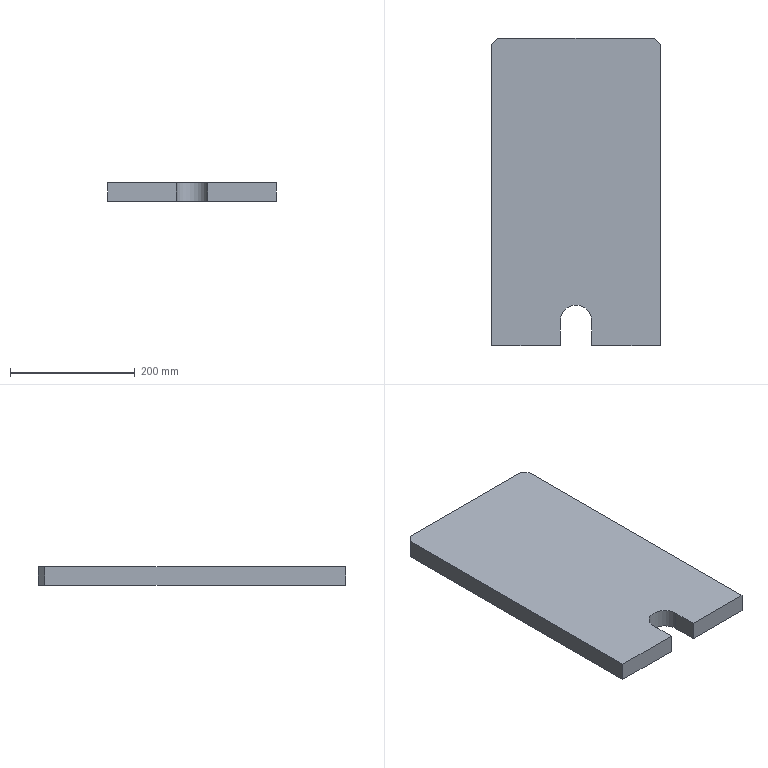Part | SolidWorks | features Extrusion 1 | 1 solid | 12 faces | box 270 x 492 x 30 mm | volume 3892748 mm3 | plane 11 | cylinder 1 | commonest cylinder face diameters 50 x1
STEP:
#1=CARTESIAN_POINT('',(0.,482.,0.));
#2=VERTEX_POINT('',#1);
#3=CARTESIAN_POINT('',(0.,0.,0.));
#4=VERTEX_POINT('',#3);
#5=CARTESIAN_POINT('',(0.,0.,0.));
#6=DIRECTION('',(0.,-1.,0.));
#7=VECTOR('',#6,1000.);
#8=LINE('',#5,#7);
#9=EDGE_CURVE('',#2,#4,#8,.T.);
#10=ORIENTED_EDGE('',*,*,#9,.T.);
#11=CARTESIAN_POINT('',(0.,0.,30.));
#12=VERTEX_POINT('',#11);
#13=CARTESIAN_POINT('',(0.,0.,30.));
#14=DIRECTION('',(0.,0.,-1.));
#15=VECTOR('',#14,1000.);
#16=LINE('',#13,#15);
#17=EDGE_CURVE('',#12,#4,#16,.T.);
#18=ORIENTED_EDGE('',*,*,#17,.F.);
#19=CARTESIAN_POINT('',(0.,482.,30.));
#20=VERTEX_POINT('',#19);
#21=CARTESIAN_POINT('',(0.,0.,30.));
#22=DIRECTION('',(0.,-1.,0.));
#23=VECTOR('',#22,1000.);
#24=LINE('',#21,#23);
#25=EDGE_CURVE('',#20,#12,#24,.T.);
#26=ORIENTED_EDGE('',*,*,#25,.F.);
#27=CARTESIAN_POINT('',(0.,482.,30.));
#28=DIRECTION('',(0.,0.,-1.));
#29=VECTOR('',#28,1000.);
#30=LINE('',#27,#29);
#31=EDGE_CURVE('',#20,#2,#30,.T.);
#32=ORIENTED_EDGE('',*,*,#31,.T.);
#33=EDGE_LOOP('',(#10,#18,#26,#32));
#34=FACE_OUTER_BOUND('',#33,.T.);
#35=CARTESIAN_POINT('',(0.,0.,30.));
#36=DIRECTION('',(1.,0.,0.));
#37=DIRECTION('',(0.,0.,-1.));
#38=AXIS2_PLACEMENT_3D('',#35,#36,#37);
#39=PLANE('',#38);
#40=ADVANCED_FACE('',(#34),#39,.F.);
#41=CARTESIAN_POINT('',(110.,0.,0.));
#42=VERTEX_POINT('',#41);
#43=CARTESIAN_POINT('',(0.,0.,0.));
#44=DIRECTION('',(1.,0.,0.));
#45=VECTOR('',#44,1000.);
#46=LINE('',#43,#45);
#47=EDGE_CURVE('',#4,#42,#46,.T.);
#48=ORIENTED_EDGE('',*,*,#47,.T.);
#49=CARTESIAN_POINT('',(110.,0.,30.));
#50=VERTEX_POINT('',#49);
#51=CARTESIAN_POINT('',(110.,0.,30.));
#52=DIRECTION('',(0.,0.,-1.));
#53=VECTOR('',#52,1000.);
#54=LINE('',#51,#53);
#55=EDGE_CURVE('',#50,#42,#54,.T.);
#56=ORIENTED_EDGE('',*,*,#55,.F.);
#57=CARTESIAN_POINT('',(0.,0.,30.));
#58=DIRECTION('',(1.,0.,0.));
#59=VECTOR('',#58,1000.);
#60=LINE('',#57,#59);
#61=EDGE_CURVE('',#12,#50,#60,.T.);
#62=ORIENTED_EDGE('',*,*,#61,.F.);
#63=ORIENTED_EDGE('',*,*,#17,.T.);
#64=EDGE_LOOP('',(#48,#56,#62,#63));
#65=FACE_OUTER_BOUND('',#64,.T.);
#66=CARTESIAN_POINT('',(0.,0.,30.));
#67=DIRECTION('',(0.,1.,0.));
#68=DIRECTION('',(0.,0.,1.));
#69=AXIS2_PLACEMENT_3D('',#66,#67,#68);
#70=PLANE('',#69);
#71=ADVANCED_FACE('',(#65),#70,.F.);
#72=CARTESIAN_POINT('',(110.,40.,0.));
#73=VERTEX_POINT('',#72);
#74=CARTESIAN_POINT('',(110.,0.,0.));
#75=DIRECTION('',(0.,1.,0.));
#76=VECTOR('',#75,1000.);
#77=LINE('',#74,#76);
#78=EDGE_CURVE('',#42,#73,#77,.T.);
#79=ORIENTED_EDGE('',*,*,#78,.T.);
#80=CARTESIAN_POINT('',(110.,40.,30.));
#81=VERTEX_POINT('',#80);
#82=CARTESIAN_POINT('',(110.,40.,30.));
#83=DIRECTION('',(0.,0.,-1.));
#84=VECTOR('',#83,1000.);
#85=LINE('',#82,#84);
#86=EDGE_CURVE('',#81,#73,#85,.T.);
#87=ORIENTED_EDGE('',*,*,#86,.F.);
#88=CARTESIAN_POINT('',(110.,0.,30.));
#89=DIRECTION('',(0.,1.,0.));
#90=VECTOR('',#89,1000.);
#91=LINE('',#88,#90);
#92=EDGE_CURVE('',#50,#81,#91,.T.);
#93=ORIENTED_EDGE('',*,*,#92,.F.);
#94=ORIENTED_EDGE('',*,*,#55,.T.);
#95=EDGE_LOOP('',(#79,#87,#93,#94));
#96=FACE_OUTER_BOUND('',#95,.T.);
#97=CARTESIAN_POINT('',(110.,0.,30.));
#98=DIRECTION('',(-1.,0.,0.));
#99=DIRECTION('',(0.,0.,1.));
#100=AXIS2_PLACEMENT_3D('',#97,#98,#99);
#101=PLANE('',#100);
#102=ADVANCED_FACE('',(#96),#101,.F.);
#103=CARTESIAN_POINT('',(160.,40.,0.));
#104=VERTEX_POINT('',#103);
#105=CARTESIAN_POINT('',(135.,40.,0.));
#106=DIRECTION('',(0.,0.,-1.));
#107=DIRECTION('',(-1.,0.,0.));
#108=AXIS2_PLACEMENT_3D('',#105,#106,#107);
#109=CIRCLE('',#108,25.);
#110=EDGE_CURVE('',#73,#104,#109,.T.);
#111=ORIENTED_EDGE('',*,*,#110,.T.);
#112=CARTESIAN_POINT('',(160.,40.,30.));
#113=VERTEX_POINT('',#112);
#114=CARTESIAN_POINT('',(160.,40.,30.));
#115=DIRECTION('',(0.,0.,-1.));
#116=VECTOR('',#115,1000.);
#117=LINE('',#114,#116);
#118=EDGE_CURVE('',#113,#104,#117,.T.);
#119=ORIENTED_EDGE('',*,*,#118,.F.);
#120=CARTESIAN_POINT('',(135.,40.,30.));
#121=DIRECTION('',(0.,0.,-1.));
#122=DIRECTION('',(-1.,0.,0.));
#123=AXIS2_PLACEMENT_3D('',#120,#121,#122);
#124=CIRCLE('',#123,25.);
#125=EDGE_CURVE('',#81,#113,#124,.T.);
#126=ORIENTED_EDGE('',*,*,#125,.F.);
#127=ORIENTED_EDGE('',*,*,#86,.T.);
#128=EDGE_LOOP('',(#111,#119,#126,#127));
#129=FACE_OUTER_BOUND('',#128,.T.);
#130=CARTESIAN_POINT('',(135.,40.,30.));
#131=DIRECTION('',(0.,0.,-1.));
#132=DIRECTION('',(-1.,0.,0.));
#133=AXIS2_PLACEMENT_3D('',#130,#131,#132);
#134=CYLINDRICAL_SURFACE('',#133,25.);
#135=ADVANCED_FACE('',(#129),#134,.F.);
#136=CARTESIAN_POINT('',(160.,0.,0.));
#137=VERTEX_POINT('',#136);
#138=CARTESIAN_POINT('',(160.,40.,0.));
#139=DIRECTION('',(0.,-1.,0.));
#140=VECTOR('',#139,1000.);
#141=LINE('',#138,#140);
#142=EDGE_CURVE('',#104,#137,#141,.T.);
#143=ORIENTED_EDGE('',*,*,#142,.T.);
#144=CARTESIAN_POINT('',(160.,0.,30.));
#145=VERTEX_POINT('',#144);
#146=CARTESIAN_POINT('',(160.,0.,30.));
#147=DIRECTION('',(0.,0.,-1.));
#148=VECTOR('',#147,1000.);
#149=LINE('',#146,#148);
#150=EDGE_CURVE('',#145,#137,#149,.T.);
#151=ORIENTED_EDGE('',*,*,#150,.F.);
#152=CARTESIAN_POINT('',(160.,40.,30.));
#153=DIRECTION('',(0.,-1.,0.));
#154=VECTOR('',#153,1000.);
#155=LINE('',#152,#154);
#156=EDGE_CURVE('',#113,#145,#155,.T.);
#157=ORIENTED_EDGE('',*,*,#156,.F.);
#158=ORIENTED_EDGE('',*,*,#118,.T.);
#159=EDGE_LOOP('',(#143,#151,#157,#158));
#160=FACE_OUTER_BOUND('',#159,.T.);
#161=CARTESIAN_POINT('',(160.,40.,30.));
#162=DIRECTION('',(1.,0.,0.));
#163=DIRECTION('',(0.,0.,-1.));
#164=AXIS2_PLACEMENT_3D('',#161,#162,#163);
#165=PLANE('',#164);
#166=ADVANCED_FACE('',(#160),#165,.F.);
#167=CARTESIAN_POINT('',(270.,0.,0.));
#168=VERTEX_POINT('',#167);
#169=CARTESIAN_POINT('',(160.,0.,0.));
#170=DIRECTION('',(1.,0.,0.));
#171=VECTOR('',#170,1000.);
#172=LINE('',#169,#171);
#173=EDGE_CURVE('',#137,#168,#172,.T.);
#174=ORIENTED_EDGE('',*,*,#173,.T.);
#175=CARTESIAN_POINT('',(270.,0.,30.));
#176=VERTEX_POINT('',#175);
#177=CARTESIAN_POINT('',(270.,0.,30.));
#178=DIRECTION('',(0.,0.,-1.));
#179=VECTOR('',#178,1000.);
#180=LINE('',#177,#179);
#181=EDGE_CURVE('',#176,#168,#180,.T.);
#182=ORIENTED_EDGE('',*,*,#181,.F.);
#183=CARTESIAN_POINT('',(160.,0.,30.));
#184=DIRECTION('',(1.,0.,0.));
#185=VECTOR('',#184,1000.);
#186=LINE('',#183,#185);
#187=EDGE_CURVE('',#145,#176,#186,.T.);
#188=ORIENTED_EDGE('',*,*,#187,.F.);
#189=ORIENTED_EDGE('',*,*,#150,.T.);
#190=EDGE_LOOP('',(#174,#182,#188,#189));
#191=FACE_OUTER_BOUND('',#190,.T.);
#192=CARTESIAN_POINT('',(160.,0.,30.));
#193=DIRECTION('',(0.,1.,0.));
#194=DIRECTION('',(0.,0.,1.));
#195=AXIS2_PLACEMENT_3D('',#192,#193,#194);
#196=PLANE('',#195);
#197=ADVANCED_FACE('',(#191),#196,.F.);
#198=CARTESIAN_POINT('',(270.,482.,0.));
#199=VERTEX_POINT('',#198);
#200=CARTESIAN_POINT('',(270.,0.,0.));
#201=DIRECTION('',(0.,1.,0.));
#202=VECTOR('',#201,1000.);
#203=LINE('',#200,#202);
#204=EDGE_CURVE('',#168,#199,#203,.T.);
#205=ORIENTED_EDGE('',*,*,#204,.T.);
#206=CARTESIAN_POINT('',(270.,482.,30.));
#207=VERTEX_POINT('',#206);
#208=CARTESIAN_POINT('',(270.,482.,30.));
#209=DIRECTION('',(0.,0.,-1.));
#210=VECTOR('',#209,1000.);
#211=LINE('',#208,#210);
#212=EDGE_CURVE('',#207,#199,#211,.T.);
#213=ORIENTED_EDGE('',*,*,#212,.F.);
#214=CARTESIAN_POINT('',(270.,0.,30.));
#215=DIRECTION('',(0.,1.,0.));
#216=VECTOR('',#215,1000.);
#217=LINE('',#214,#216);
#218=EDGE_CURVE('',#176,#207,#217,.T.);
#219=ORIENTED_EDGE('',*,*,#218,.F.);
#220=ORIENTED_EDGE('',*,*,#181,.T.);
#221=EDGE_LOOP('',(#205,#213,#219,#220));
#222=FACE_OUTER_BOUND('',#221,.T.);
#223=CARTESIAN_POINT('',(270.,0.,30.));
#224=DIRECTION('',(-1.,0.,0.));
#225=DIRECTION('',(0.,0.,1.));
#226=AXIS2_PLACEMENT_3D('',#223,#224,#225);
#227=PLANE('',#226);
#228=ADVANCED_FACE('',(#222),#227,.F.);
#229=CARTESIAN_POINT('',(260.,492.,0.));
#230=VERTEX_POINT('',#229);
#231=CARTESIAN_POINT('',(260.,492.,0.));
#232=DIRECTION('',(-0.7071,0.7071,0.));
#233=VECTOR('',#232,1000.);
#234=LINE('',#231,#233);
#235=EDGE_CURVE('',#199,#230,#234,.T.);
#236=ORIENTED_EDGE('',*,*,#235,.T.);
#237=CARTESIAN_POINT('',(260.,492.,30.));
#238=VERTEX_POINT('',#237);
#239=CARTESIAN_POINT('',(260.,492.,30.));
#240=DIRECTION('',(0.,0.,-1.));
#241=VECTOR('',#240,1000.);
#242=LINE('',#239,#241);
#243=EDGE_CURVE('',#238,#230,#242,.T.);
#244=ORIENTED_EDGE('',*,*,#243,.F.);
#245=CARTESIAN_POINT('',(260.,492.,30.));
#246=DIRECTION('',(-0.7071,0.7071,0.));
#247=VECTOR('',#246,1000.);
#248=LINE('',#245,#247);
#249=EDGE_CURVE('',#207,#238,#248,.T.);
#250=ORIENTED_EDGE('',*,*,#249,.F.);
#251=ORIENTED_EDGE('',*,*,#212,.T.);
#252=EDGE_LOOP('',(#236,#244,#250,#251));
#253=FACE_OUTER_BOUND('',#252,.T.);
#254=CARTESIAN_POINT('',(260.,492.,30.));
#255=DIRECTION('',(-0.7071,-0.7071,0.));
#256=DIRECTION('',(0.7071,-0.7071,0.));
#257=AXIS2_PLACEMENT_3D('',#254,#255,#256);
#258=PLANE('',#257);
#259=ADVANCED_FACE('',(#253),#258,.F.);
#260=CARTESIAN_POINT('',(10.,492.,0.));
#261=VERTEX_POINT('',#260);
#262=CARTESIAN_POINT('',(10.,492.,0.));
#263=DIRECTION('',(-1.,0.,0.));
#264=VECTOR('',#263,1000.);
#265=LINE('',#262,#264);
#266=EDGE_CURVE('',#230,#261,#265,.T.);
#267=ORIENTED_EDGE('',*,*,#266,.T.);
#268=CARTESIAN_POINT('',(10.,492.,30.));
#269=VERTEX_POINT('',#268);
#270=CARTESIAN_POINT('',(10.,492.,30.));
#271=DIRECTION('',(0.,0.,-1.));
#272=VECTOR('',#271,1000.);
#273=LINE('',#270,#272);
#274=EDGE_CURVE('',#269,#261,#273,.T.);
#275=ORIENTED_EDGE('',*,*,#274,.F.);
#276=CARTESIAN_POINT('',(10.,492.,30.));
#277=DIRECTION('',(-1.,0.,0.));
#278=VECTOR('',#277,1000.);
#279=LINE('',#276,#278);
#280=EDGE_CURVE('',#238,#269,#279,.T.);
#281=ORIENTED_EDGE('',*,*,#280,.F.);
#282=ORIENTED_EDGE('',*,*,#243,.T.);
#283=EDGE_LOOP('',(#267,#275,#281,#282));
#284=FACE_OUTER_BOUND('',#283,.T.);
#285=CARTESIAN_POINT('',(10.,492.,30.));
#286=DIRECTION('',(0.,-1.,0.));
#287=DIRECTION('',(1.,0.,0.));
#288=AXIS2_PLACEMENT_3D('',#285,#286,#287);
#289=PLANE('',#288);
#290=ADVANCED_FACE('',(#284),#289,.F.);
#291=CARTESIAN_POINT('',(0.,482.,0.));
#292=DIRECTION('',(-0.7071,-0.7071,0.));
#293=VECTOR('',#292,1000.);
#294=LINE('',#291,#293);
#295=EDGE_CURVE('',#261,#2,#294,.T.);
#296=ORIENTED_EDGE('',*,*,#295,.T.);
#297=ORIENTED_EDGE('',*,*,#31,.F.);
#298=CARTESIAN_POINT('',(0.,482.,30.));
#299=DIRECTION('',(-0.7071,-0.7071,0.));
#300=VECTOR('',#299,1000.);
#301=LINE('',#298,#300);
#302=EDGE_CURVE('',#269,#20,#301,.T.);
#303=ORIENTED_EDGE('',*,*,#302,.F.);
#304=ORIENTED_EDGE('',*,*,#274,.T.);
#305=EDGE_LOOP('',(#296,#297,#303,#304));
#306=FACE_OUTER_BOUND('',#305,.T.);
#307=CARTESIAN_POINT('',(0.,482.,30.));
#308=DIRECTION('',(0.7071,-0.7071,0.));
#309=DIRECTION('',(0.7071,0.7071,0.));
#310=AXIS2_PLACEMENT_3D('',#307,#308,#309);
#311=PLANE('',#310);
#312=ADVANCED_FACE('',(#306),#311,.F.);
#313=ORIENTED_EDGE('',*,*,#25,.T.);
#314=ORIENTED_EDGE('',*,*,#61,.T.);
#315=ORIENTED_EDGE('',*,*,#92,.T.);
#316=ORIENTED_EDGE('',*,*,#125,.T.);
#317=ORIENTED_EDGE('',*,*,#156,.T.);
#318=ORIENTED_EDGE('',*,*,#187,.T.);
#319=ORIENTED_EDGE('',*,*,#218,.T.);
#320=ORIENTED_EDGE('',*,*,#249,.T.);
#321=ORIENTED_EDGE('',*,*,#280,.T.);
#322=ORIENTED_EDGE('',*,*,#302,.T.);
#323=EDGE_LOOP('',(#313,#314,#315,#316,#317,#318,#319,#320,#321,#322));
#324=FACE_OUTER_BOUND('',#323,.T.);
#325=CARTESIAN_POINT('',(135.,40.,30.));
#326=DIRECTION('',(0.,0.,-1.));
#327=DIRECTION('',(-1.,0.,0.));
#328=AXIS2_PLACEMENT_3D('',#325,#326,#327);
#329=PLANE('',#328);
#330=ADVANCED_FACE('',(#324),#329,.F.);
#331=ORIENTED_EDGE('',*,*,#9,.F.);
#332=ORIENTED_EDGE('',*,*,#295,.F.);
#333=ORIENTED_EDGE('',*,*,#266,.F.);
#334=ORIENTED_EDGE('',*,*,#235,.F.);
#335=ORIENTED_EDGE('',*,*,#204,.F.);
#336=ORIENTED_EDGE('',*,*,#173,.F.);
#337=ORIENTED_EDGE('',*,*,#142,.F.);
#338=ORIENTED_EDGE('',*,*,#110,.F.);
#339=ORIENTED_EDGE('',*,*,#78,.F.);
#340=ORIENTED_EDGE('',*,*,#47,.F.);
#341=EDGE_LOOP('',(#331,#332,#333,#334,#335,#336,#337,#338,#339,#340));
#342=FACE_OUTER_BOUND('',#341,.T.);
#343=CARTESIAN_POINT('',(135.,40.,0.));
#344=DIRECTION('',(0.,0.,-1.));
#345=DIRECTION('',(-1.,0.,0.));
#346=AXIS2_PLACEMENT_3D('',#343,#344,#345);
#347=PLANE('',#346);
#348=ADVANCED_FACE('',(#342),#347,.T.);
#349=CLOSED_SHELL('',(#40,#71,#102,#135,#166,#197,#228,#259,#290,#312,#330,#348));
#350=MANIFOLD_SOLID_BREP('',#349);
#351=CARTESIAN_POINT('',(0.,0.,0.));
#352=DIRECTION('',(0.,0.,1.));
#353=DIRECTION('',(1.,0.,0.));
#354=AXIS2_PLACEMENT_3D('',#351,#352,#353);
#355=(LENGTH_UNIT()NAMED_UNIT(*)SI_UNIT(.MILLI.,.METRE.));
#356=UNCERTAINTY_MEASURE_WITH_UNIT(LENGTH_MEASURE(0.00001),#355,'','');
#357=(NAMED_UNIT(*)PLANE_ANGLE_UNIT()SI_UNIT($,.RADIAN.));
#358=(NAMED_UNIT(*)SI_UNIT($,.STERADIAN.)SOLID_ANGLE_UNIT());
#359=(GEOMETRIC_REPRESENTATION_CONTEXT(3)GLOBAL_UNCERTAINTY_ASSIGNED_CONTEXT((#356))GLOBAL_UNIT_ASSIGNED_CONTEXT((#355,#357,#358))REPRESENTATION_CONTEXT('',''));
#360=ADVANCED_BREP_SHAPE_REPRESENTATION('',(#350,#354),#359);